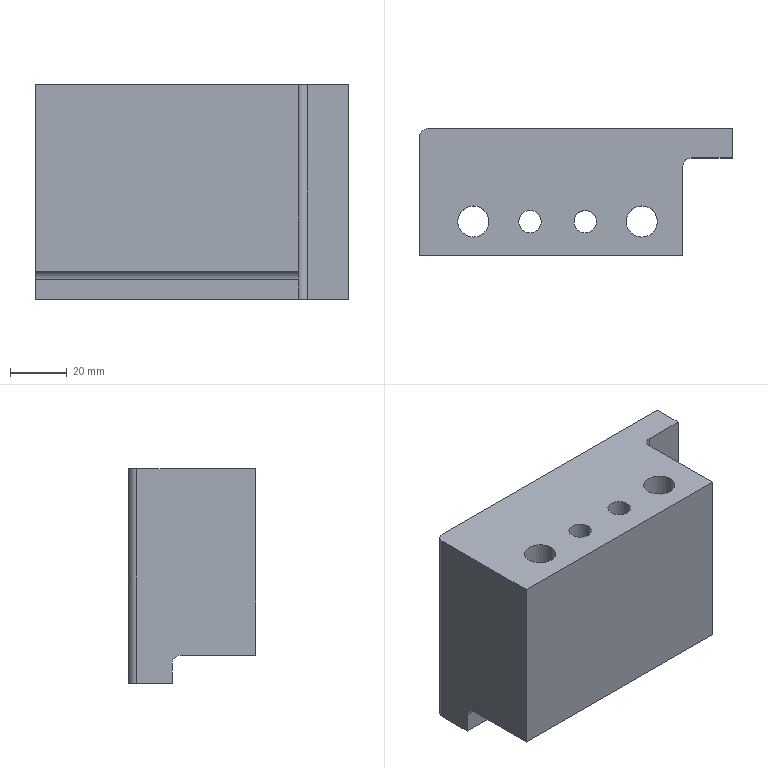Part | NX | features solid 2 | 1 solid | 25 faces | box 110.531 x 45 x 76 mm | volume 273418 mm3 | plane 14 | cylinder 11 | commonest cylinder face diameters 6 x3 8 x2 10.505 x2 11 x2 17 x2
STEP:
#1=CARTESIAN_POINT('',(667.977,-186.119,32.999));
#2=VERTEX_POINT('',#1);
#3=CARTESIAN_POINT('',(667.977,-180.619,32.999));
#4=DIRECTION('',(0.000000053,-0.000000517,1.));
#5=DIRECTION('',(0.,-1.,-0.000000517));
#6=AXIS2_PLACEMENT_3D('',#3,#4,#5);
#7=CIRCLE('',#6,5.5);
#8=EDGE_CURVE('',#2,#2,#7,.F.);
#9=ORIENTED_EDGE('',*,*,#8,.T.);
#10=EDGE_LOOP('',(#9));
#11=FACE_BOUND('',#10,.T.);
#12=CARTESIAN_POINT('',(647.977,-184.619,32.999));
#13=VERTEX_POINT('',#12);
#14=CARTESIAN_POINT('',(647.977,-180.619,32.999));
#15=DIRECTION('',(-0.000000053,0.000000517,-1.));
#16=DIRECTION('',(0.,-1.,-0.000000517));
#17=AXIS2_PLACEMENT_3D('',#14,#15,#16);
#18=CIRCLE('',#17,4.);
#19=EDGE_CURVE('',#13,#13,#18,.T.);
#20=ORIENTED_EDGE('',*,*,#19,.T.);
#21=EDGE_LOOP('',(#20));
#22=FACE_BOUND('',#21,.T.);
#23=CARTESIAN_POINT('',(628.446,-184.619,32.999));
#24=VERTEX_POINT('',#23);
#25=CARTESIAN_POINT('',(628.446,-180.619,32.999));
#26=DIRECTION('',(-0.000000053,0.000000517,-1.));
#27=DIRECTION('',(0.,-1.,-0.000000517));
#28=AXIS2_PLACEMENT_3D('',#25,#26,#27);
#29=CIRCLE('',#28,4.);
#30=EDGE_CURVE('',#24,#24,#29,.T.);
#31=ORIENTED_EDGE('',*,*,#30,.T.);
#32=EDGE_LOOP('',(#31));
#33=FACE_BOUND('',#32,.T.);
#34=CARTESIAN_POINT('',(608.446,-186.119,32.999));
#35=VERTEX_POINT('',#34);
#36=CARTESIAN_POINT('',(608.446,-180.619,32.999));
#37=DIRECTION('',(0.000000053,-0.000000517,1.));
#38=DIRECTION('',(0.,-1.,-0.000000517));
#39=AXIS2_PLACEMENT_3D('',#36,#37,#38);
#40=CIRCLE('',#39,5.5);
#41=EDGE_CURVE('',#35,#35,#40,.F.);
#42=ORIENTED_EDGE('',*,*,#41,.T.);
#43=EDGE_LOOP('',(#42));
#44=FACE_BOUND('',#43,.T.);
#45=CARTESIAN_POINT('',(682.498,-161.1,32.999));
#46=VERTEX_POINT('',#45);
#47=CARTESIAN_POINT('',(682.498,-192.619,32.999));
#48=VERTEX_POINT('',#47);
#49=CARTESIAN_POINT('',(682.498,-187.619,32.999));
#50=DIRECTION('',(0.,1.,0.000000517));
#51=VECTOR('',#50,1000.);
#52=LINE('',#49,#51);
#53=EDGE_CURVE('',#46,#48,#52,.F.);
#54=ORIENTED_EDGE('',*,*,#53,.F.);
#55=CARTESIAN_POINT('',(685.498,-158.1,32.999));
#56=VERTEX_POINT('',#55);
#57=CARTESIAN_POINT('',(685.498,-161.1,32.999));
#58=DIRECTION('',(0.000000053,-0.000000517,1.));
#59=DIRECTION('',(-0.01202,0.9999,0.000000518));
#60=AXIS2_PLACEMENT_3D('',#57,#58,#59);
#61=ELLIPSE('',#60,3.,3.);
#62=EDGE_CURVE('',#46,#56,#61,.F.);
#63=ORIENTED_EDGE('',*,*,#62,.T.);
#64=CARTESIAN_POINT('',(699.977,-158.1,32.999));
#65=VERTEX_POINT('',#64);
#66=CARTESIAN_POINT('',(699.977,-158.1,32.999));
#67=DIRECTION('',(-1.,0.,0.000000053));
#68=VECTOR('',#67,1000.);
#69=LINE('',#66,#68);
#70=EDGE_CURVE('',#65,#56,#69,.T.);
#71=ORIENTED_EDGE('',*,*,#70,.F.);
#72=CARTESIAN_POINT('',(699.977,-147.619,32.999));
#73=VERTEX_POINT('',#72);
#74=CARTESIAN_POINT('',(699.977,-187.619,32.999));
#75=DIRECTION('',(0.,1.,0.000000517));
#76=VECTOR('',#75,1000.);
#77=LINE('',#74,#76);
#78=EDGE_CURVE('',#65,#73,#77,.T.);
#79=ORIENTED_EDGE('',*,*,#78,.T.);
#80=CARTESIAN_POINT('',(592.446,-147.619,32.999));
#81=VERTEX_POINT('',#80);
#82=CARTESIAN_POINT('',(699.977,-147.619,32.999));
#83=DIRECTION('',(-1.,0.,0.000000053));
#84=VECTOR('',#83,1000.);
#85=LINE('',#82,#84);
#86=EDGE_CURVE('',#81,#73,#85,.F.);
#87=ORIENTED_EDGE('',*,*,#86,.F.);
#88=CARTESIAN_POINT('',(589.446,-150.619,32.999));
#89=VERTEX_POINT('',#88);
#90=CARTESIAN_POINT('',(592.446,-150.619,32.999));
#91=DIRECTION('',(0.000000053,-0.000000517,1.));
#92=DIRECTION('',(0.,1.,0.000000517));
#93=AXIS2_PLACEMENT_3D('',#90,#91,#92);
#94=CIRCLE('',#93,3.);
#95=EDGE_CURVE('',#89,#81,#94,.F.);
#96=ORIENTED_EDGE('',*,*,#95,.F.);
#97=CARTESIAN_POINT('',(589.446,-192.619,32.999));
#98=VERTEX_POINT('',#97);
#99=CARTESIAN_POINT('',(589.446,-177.619,32.999));
#100=DIRECTION('',(0.,1.,0.000000517));
#101=VECTOR('',#100,1000.);
#102=LINE('',#99,#101);
#103=EDGE_CURVE('',#89,#98,#102,.F.);
#104=ORIENTED_EDGE('',*,*,#103,.T.);
#105=CARTESIAN_POINT('',(699.977,-192.619,32.999));
#106=DIRECTION('',(-1.,0.,0.000000053));
#107=VECTOR('',#106,1000.);
#108=LINE('',#105,#107);
#109=EDGE_CURVE('',#98,#48,#108,.F.);
#110=ORIENTED_EDGE('',*,*,#109,.T.);
#111=EDGE_LOOP('',(#54,#63,#71,#79,#87,#96,#104,#110));
#112=FACE_BOUND('',#111,.T.);
#113=CARTESIAN_POINT('',(699.977,-187.619,32.999));
#114=DIRECTION('',(0.000000053,-0.000000517,1.));
#115=DIRECTION('',(1.,0.,-0.000000053));
#116=AXIS2_PLACEMENT_3D('',#113,#114,#115);
#117=PLANE('',#116);
#118=ADVANCED_FACE('',(#11,#22,#33,#44,#112),#117,.T.);
#119=CARTESIAN_POINT('',(682.498,-163.1,-43.001));
#120=VERTEX_POINT('',#119);
#121=CARTESIAN_POINT('',(682.498,-163.1,-36.001));
#122=VERTEX_POINT('',#121);
#123=CARTESIAN_POINT('',(682.498,-163.1,-5.001));
#124=DIRECTION('',(0.,0.000003911,1.));
#125=VECTOR('',#124,1000.);
#126=LINE('',#123,#125);
#127=EDGE_CURVE('',#120,#122,#126,.T.);
#128=ORIENTED_EDGE('',*,*,#127,.T.);
#129=CARTESIAN_POINT('',(589.446,-163.1,-36.001));
#130=VERTEX_POINT('',#129);
#131=CARTESIAN_POINT('',(589.446,-163.1,-36.001));
#132=DIRECTION('',(1.,0.,-0.000000053));
#133=VECTOR('',#132,1000.);
#134=LINE('',#131,#133);
#135=EDGE_CURVE('',#122,#130,#134,.F.);
#136=ORIENTED_EDGE('',*,*,#135,.T.);
#137=CARTESIAN_POINT('',(589.446,-163.1,-43.001));
#138=VERTEX_POINT('',#137);
#139=CARTESIAN_POINT('',(589.446,-163.1,-5.001));
#140=DIRECTION('',(-0.000000053,-0.000003911,-1.));
#141=VECTOR('',#140,1000.);
#142=LINE('',#139,#141);
#143=EDGE_CURVE('',#130,#138,#142,.T.);
#144=ORIENTED_EDGE('',*,*,#143,.T.);
#145=CARTESIAN_POINT('',(574.977,-163.1,-43.001));
#146=DIRECTION('',(-1.,0.,0.000000053));
#147=VECTOR('',#146,1000.);
#148=LINE('',#145,#147);
#149=EDGE_CURVE('',#120,#138,#148,.T.);
#150=ORIENTED_EDGE('',*,*,#149,.F.);
#151=EDGE_LOOP('',(#128,#136,#144,#150));
#152=FACE_BOUND('',#151,.T.);
#153=CARTESIAN_POINT('',(704.737,-163.1,-5.001));
#154=DIRECTION('',(0.,-1.,0.000003911));
#155=DIRECTION('',(0.,-0.000003911,-1.));
#156=AXIS2_PLACEMENT_3D('',#153,#154,#155);
#157=PLANE('',#156);
#158=ADVANCED_FACE('',(#152),#157,.T.);
#159=ORIENTED_EDGE('',*,*,#86,.T.);
#160=CARTESIAN_POINT('',(699.977,-147.619,-43.001));
#161=VERTEX_POINT('',#160);
#162=CARTESIAN_POINT('',(699.977,-147.619,56.368));
#163=DIRECTION('',(0.000000053,-0.000000517,1.));
#164=VECTOR('',#163,1000.);
#165=LINE('',#162,#164);
#166=EDGE_CURVE('',#161,#73,#165,.T.);
#167=ORIENTED_EDGE('',*,*,#166,.F.);
#168=CARTESIAN_POINT('',(592.446,-147.619,-43.001));
#169=VERTEX_POINT('',#168);
#170=CARTESIAN_POINT('',(574.977,-147.619,-43.001));
#171=DIRECTION('',(1.,0.,-0.000000053));
#172=VECTOR('',#171,1000.);
#173=LINE('',#170,#172);
#174=EDGE_CURVE('',#169,#161,#173,.T.);
#175=ORIENTED_EDGE('',*,*,#174,.F.);
#176=CARTESIAN_POINT('',(592.446,-147.619,56.368));
#177=DIRECTION('',(-0.000000053,0.000000517,-1.));
#178=VECTOR('',#177,1000.);
#179=LINE('',#176,#178);
#180=EDGE_CURVE('',#81,#169,#179,.T.);
#181=ORIENTED_EDGE('',*,*,#180,.F.);
#182=EDGE_LOOP('',(#159,#167,#175,#181));
#183=FACE_BOUND('',#182,.T.);
#184=CARTESIAN_POINT('',(583.446,-147.619,56.368));
#185=DIRECTION('',(0.,-1.,-0.000000517));
#186=DIRECTION('',(-0.000000053,0.000000517,-1.));
#187=AXIS2_PLACEMENT_3D('',#184,#185,#186);
#188=PLANE('',#187);
#189=ADVANCED_FACE('',(#183),#188,.F.);
#190=ORIENTED_EDGE('',*,*,#174,.T.);
#191=CARTESIAN_POINT('',(699.977,-158.1,-43.001));
#192=VERTEX_POINT('',#191);
#193=CARTESIAN_POINT('',(699.977,-110.331,-43.001));
#194=DIRECTION('',(0.,-1.,-0.000000517));
#195=VECTOR('',#194,1000.);
#196=LINE('',#193,#195);
#197=EDGE_CURVE('',#161,#192,#196,.T.);
#198=ORIENTED_EDGE('',*,*,#197,.T.);
#199=CARTESIAN_POINT('',(685.498,-158.1,-43.001));
#200=VERTEX_POINT('',#199);
#201=CARTESIAN_POINT('',(574.977,-158.1,-43.001));
#202=DIRECTION('',(-1.,0.,0.000000053));
#203=VECTOR('',#202,1000.);
#204=LINE('',#201,#203);
#205=EDGE_CURVE('',#192,#200,#204,.T.);
#206=ORIENTED_EDGE('',*,*,#205,.T.);
#207=CARTESIAN_POINT('',(682.498,-161.1,-43.001));
#208=VERTEX_POINT('',#207);
#209=CARTESIAN_POINT('',(685.498,-161.1,-43.001));
#210=DIRECTION('',(-0.000000053,0.000000517,-1.));
#211=DIRECTION('',(-0.01202,0.9999,0.000000518));
#212=AXIS2_PLACEMENT_3D('',#209,#210,#211);
#213=ELLIPSE('',#212,3.,3.);
#214=EDGE_CURVE('',#200,#208,#213,.F.);
#215=ORIENTED_EDGE('',*,*,#214,.T.);
#216=CARTESIAN_POINT('',(682.498,-110.331,-43.001));
#217=DIRECTION('',(0.,-1.,-0.000000517));
#218=VECTOR('',#217,1000.);
#219=LINE('',#216,#218);
#220=EDGE_CURVE('',#208,#120,#219,.T.);
#221=ORIENTED_EDGE('',*,*,#220,.T.);
#222=ORIENTED_EDGE('',*,*,#149,.T.);
#223=CARTESIAN_POINT('',(589.446,-150.619,-43.001));
#224=VERTEX_POINT('',#223);
#225=CARTESIAN_POINT('',(589.446,-110.331,-43.001));
#226=DIRECTION('',(0.,1.,0.000000517));
#227=VECTOR('',#226,1000.);
#228=LINE('',#225,#227);
#229=EDGE_CURVE('',#138,#224,#228,.T.);
#230=ORIENTED_EDGE('',*,*,#229,.T.);
#231=CARTESIAN_POINT('',(592.446,-150.619,-43.001));
#232=DIRECTION('',(-0.000000053,0.000000517,-1.));
#233=DIRECTION('',(0.,-1.,-0.000000517));
#234=AXIS2_PLACEMENT_3D('',#231,#232,#233);
#235=CIRCLE('',#234,3.);
#236=EDGE_CURVE('',#169,#224,#235,.F.);
#237=ORIENTED_EDGE('',*,*,#236,.F.);
#238=EDGE_LOOP('',(#190,#198,#206,#215,#221,#222,#230,#237));
#239=FACE_BOUND('',#238,.T.);
#240=CARTESIAN_POINT('',(574.977,-110.331,-43.001));
#241=DIRECTION('',(-0.000000053,0.000000517,-1.));
#242=DIRECTION('',(1.,0.,-0.000000053));
#243=AXIS2_PLACEMENT_3D('',#240,#241,#242);
#244=PLANE('',#243);
#245=ADVANCED_FACE('',(#239),#244,.T.);
#246=CARTESIAN_POINT('',(589.446,-192.619,-33.001));
#247=VERTEX_POINT('',#246);
#248=CARTESIAN_POINT('',(589.446,-166.1,-33.001));
#249=VERTEX_POINT('',#248);
#250=CARTESIAN_POINT('',(589.446,-110.331,-33.001));
#251=DIRECTION('',(0.,1.,0.000000517));
#252=VECTOR('',#251,1000.);
#253=LINE('',#250,#252);
#254=EDGE_CURVE('',#247,#249,#253,.T.);
#255=ORIENTED_EDGE('',*,*,#254,.T.);
#256=CARTESIAN_POINT('',(682.498,-166.1,-33.001));
#257=VERTEX_POINT('',#256);
#258=CARTESIAN_POINT('',(682.498,-166.1,-33.001));
#259=DIRECTION('',(1.,0.,-0.000000053));
#260=VECTOR('',#259,1000.);
#261=LINE('',#258,#260);
#262=EDGE_CURVE('',#249,#257,#261,.T.);
#263=ORIENTED_EDGE('',*,*,#262,.T.);
#264=CARTESIAN_POINT('',(682.498,-192.619,-33.001));
#265=VERTEX_POINT('',#264);
#266=CARTESIAN_POINT('',(682.498,-110.331,-33.001));
#267=DIRECTION('',(0.,-1.,-0.000000517));
#268=VECTOR('',#267,1000.);
#269=LINE('',#266,#268);
#270=EDGE_CURVE('',#257,#265,#269,.T.);
#271=ORIENTED_EDGE('',*,*,#270,.T.);
#272=CARTESIAN_POINT('',(574.977,-192.619,-33.001));
#273=DIRECTION('',(-1.,0.,0.000000053));
#274=VECTOR('',#273,1000.);
#275=LINE('',#272,#274);
#276=EDGE_CURVE('',#265,#247,#275,.T.);
#277=ORIENTED_EDGE('',*,*,#276,.T.);
#278=EDGE_LOOP('',(#255,#263,#271,#277));
#279=FACE_BOUND('',#278,.T.);
#280=CARTESIAN_POINT('',(608.446,-172.119,-33.001));
#281=VERTEX_POINT('',#280);
#282=CARTESIAN_POINT('',(608.446,-180.619,-33.001));
#283=DIRECTION('',(-0.000000053,0.000000517,-1.));
#284=DIRECTION('',(0.,1.,0.000000517));
#285=AXIS2_PLACEMENT_3D('',#282,#283,#284);
#286=CIRCLE('',#285,8.5);
#287=EDGE_CURVE('',#281,#281,#286,.T.);
#288=ORIENTED_EDGE('',*,*,#287,.F.);
#289=EDGE_LOOP('',(#288));
#290=FACE_BOUND('',#289,.T.);
#291=CARTESIAN_POINT('',(628.446,-175.366,-33.001));
#292=VERTEX_POINT('',#291);
#293=CARTESIAN_POINT('',(627.378,-175.439,-33.001));
#294=CARTESIAN_POINT('',(628.411,-175.332,-33.001));
#295=CARTESIAN_POINT('',(629.442,-175.429,-33.001));
#296=CARTESIAN_POINT('',(630.419,-175.714,-33.001));
#297=CARTESIAN_POINT('',(631.337,-176.193,-33.001));
#298=CARTESIAN_POINT('',(632.145,-176.842,-33.001));
#299=CARTESIAN_POINT('',(632.811,-177.636,-33.001));
#300=CARTESIAN_POINT('',(633.309,-178.545,-33.001));
#301=CARTESIAN_POINT('',(633.62,-179.533,-33.001));
#302=CARTESIAN_POINT('',(633.732,-180.564,-33.001));
#303=CARTESIAN_POINT('',(633.641,-181.596,-33.001));
#304=CARTESIAN_POINT('',(633.351,-182.591,-33.001));
#305=CARTESIAN_POINT('',(632.872,-183.51,-33.001));
#306=CARTESIAN_POINT('',(632.223,-184.318,-33.001));
#307=CARTESIAN_POINT('',(631.428,-184.983,-33.001));
#308=CARTESIAN_POINT('',(630.52,-185.481,-33.001));
#309=CARTESIAN_POINT('',(629.531,-185.792,-33.001));
#310=CARTESIAN_POINT('',(628.501,-185.905,-33.001));
#311=CARTESIAN_POINT('',(627.469,-185.814,-33.001));
#312=CARTESIAN_POINT('',(626.474,-185.523,-33.001));
#313=CARTESIAN_POINT('',(625.555,-185.044,-33.001));
#314=CARTESIAN_POINT('',(624.747,-184.395,-33.001));
#315=CARTESIAN_POINT('',(624.081,-183.601,-33.001));
#316=CARTESIAN_POINT('',(623.583,-182.692,-33.001));
#317=CARTESIAN_POINT('',(623.272,-181.704,-33.001));
#318=CARTESIAN_POINT('',(623.16,-180.673,-33.001));
#319=CARTESIAN_POINT('',(623.251,-179.641,-33.001));
#320=CARTESIAN_POINT('',(623.541,-178.646,-33.001));
#321=CARTESIAN_POINT('',(624.02,-177.727,-33.001));
#322=CARTESIAN_POINT('',(624.669,-176.919,-33.001));
#323=CARTESIAN_POINT('',(625.464,-176.254,-33.001));
#324=CARTESIAN_POINT('',(626.373,-175.756,-33.001));
#325=CARTESIAN_POINT('',(627.378,-175.439,-33.001));
#326=CARTESIAN_POINT('',(628.411,-175.332,-33.001));
#327=CARTESIAN_POINT('',(629.442,-175.429,-33.001));
#328=B_SPLINE_CURVE_WITH_KNOTS('',3,(#293,#294,#295,#296,#297,#298,#299,#300,#301,#302,#303,#304,#305,#306,#307,#308,#309,#310,#311,#312,#313,#314,#315,#316,#317,#318,#319,#320,#321,#322,#323,#324,#325,#326,#327),.UNSPECIFIED.,.T.,.F.,(1,1,1,1,1,1,1,1,1,1,1,1,1,1,1,1,1,1,1,1,1,1,1,1,1,1,1,1,1,1,1,1,1,1,1,1,1,1,1),(-0.09539,-0.06414,-0.03289,0.,0.02969,0.06086,0.09211,0.1234,0.1546,0.1859,0.2171,0.2484,0.2796,0.3109,0.3421,0.3734,0.4046,0.4359,0.4671,0.4984,0.5296,0.5609,0.5921,0.6234,0.6546,0.6859,0.7171,0.7484,0.7796,0.8109,0.8421,0.8734,0.9046,0.9359,0.9671,1.,1.03,1.061,1.092),.UNSPECIFIED.);
#329=EDGE_CURVE('',#292,#292,#328,.T.);
#330=ORIENTED_EDGE('',*,*,#329,.F.);
#331=EDGE_LOOP('',(#330));
#332=FACE_BOUND('',#331,.T.);
#333=CARTESIAN_POINT('',(647.977,-175.366,-33.001));
#334=VERTEX_POINT('',#333);
#335=CARTESIAN_POINT('',(649.045,-175.439,-33.001));
#336=CARTESIAN_POINT('',(648.012,-175.332,-33.001));
#337=CARTESIAN_POINT('',(646.981,-175.429,-33.001));
#338=CARTESIAN_POINT('',(646.004,-175.714,-33.001));
#339=CARTESIAN_POINT('',(645.086,-176.193,-33.001));
#340=CARTESIAN_POINT('',(644.278,-176.842,-33.001));
#341=CARTESIAN_POINT('',(643.613,-177.636,-33.001));
#342=CARTESIAN_POINT('',(643.115,-178.545,-33.001));
#343=CARTESIAN_POINT('',(642.804,-179.533,-33.001));
#344=CARTESIAN_POINT('',(642.691,-180.564,-33.001));
#345=CARTESIAN_POINT('',(642.782,-181.596,-33.001));
#346=CARTESIAN_POINT('',(643.073,-182.591,-33.001));
#347=CARTESIAN_POINT('',(643.552,-183.51,-33.001));
#348=CARTESIAN_POINT('',(644.201,-184.318,-33.001));
#349=CARTESIAN_POINT('',(644.995,-184.983,-33.001));
#350=CARTESIAN_POINT('',(645.904,-185.481,-33.001));
#351=CARTESIAN_POINT('',(646.892,-185.792,-33.001));
#352=CARTESIAN_POINT('',(647.923,-185.905,-33.001));
#353=CARTESIAN_POINT('',(648.955,-185.814,-33.001));
#354=CARTESIAN_POINT('',(649.95,-185.523,-33.001));
#355=CARTESIAN_POINT('',(650.869,-185.044,-33.001));
#356=CARTESIAN_POINT('',(651.676,-184.395,-33.001));
#357=CARTESIAN_POINT('',(652.342,-183.601,-33.001));
#358=CARTESIAN_POINT('',(652.84,-182.692,-33.001));
#359=CARTESIAN_POINT('',(653.151,-181.703,-33.001));
#360=CARTESIAN_POINT('',(653.263,-180.673,-33.001));
#361=CARTESIAN_POINT('',(653.173,-179.641,-33.001));
#362=CARTESIAN_POINT('',(652.882,-178.646,-33.001));
#363=CARTESIAN_POINT('',(652.403,-177.727,-33.001));
#364=CARTESIAN_POINT('',(651.754,-176.919,-33.001));
#365=CARTESIAN_POINT('',(650.96,-176.254,-33.001));
#366=CARTESIAN_POINT('',(650.051,-175.756,-33.001));
#367=CARTESIAN_POINT('',(649.045,-175.439,-33.001));
#368=CARTESIAN_POINT('',(648.012,-175.332,-33.001));
#369=CARTESIAN_POINT('',(646.981,-175.429,-33.001));
#370=B_SPLINE_CURVE_WITH_KNOTS('',3,(#335,#336,#337,#338,#339,#340,#341,#342,#343,#344,#345,#346,#347,#348,#349,#350,#351,#352,#353,#354,#355,#356,#357,#358,#359,#360,#361,#362,#363,#364,#365,#366,#367,#368,#369),.UNSPECIFIED.,.T.,.F.,(1,1,1,1,1,1,1,1,1,1,1,1,1,1,1,1,1,1,1,1,1,1,1,1,1,1,1,1,1,1,1,1,1,1,1,1,1,1,1),(-0.09539,-0.06414,-0.03289,0.,0.02969,0.06086,0.09211,0.1234,0.1546,0.1859,0.2171,0.2484,0.2796,0.3109,0.3421,0.3734,0.4046,0.4359,0.4671,0.4984,0.5296,0.5609,0.5921,0.6234,0.6546,0.6859,0.7171,0.7484,0.7796,0.8109,0.8421,0.8734,0.9046,0.9359,0.9671,1.,1.03,1.061,1.092),.UNSPECIFIED.);
#371=EDGE_CURVE('',#334,#334,#370,.F.);
#372=ORIENTED_EDGE('',*,*,#371,.F.);
#373=EDGE_LOOP('',(#372));
#374=FACE_BOUND('',#373,.T.);
#375=CARTESIAN_POINT('',(667.977,-172.119,-33.001));
#376=VERTEX_POINT('',#375);
#377=CARTESIAN_POINT('',(667.977,-180.619,-33.001));
#378=DIRECTION('',(-0.000000053,0.000000517,-1.));
#379=DIRECTION('',(0.,1.,0.000000517));
#380=AXIS2_PLACEMENT_3D('',#377,#378,#379);
#381=CIRCLE('',#380,8.5);
#382=EDGE_CURVE('',#376,#376,#381,.T.);
#383=ORIENTED_EDGE('',*,*,#382,.F.);
#384=EDGE_LOOP('',(#383));
#385=FACE_BOUND('',#384,.T.);
#386=CARTESIAN_POINT('',(574.977,-110.331,-33.001));
#387=DIRECTION('',(-0.000000053,0.000000517,-1.));
#388=DIRECTION('',(1.,0.,-0.000000053));
#389=AXIS2_PLACEMENT_3D('',#386,#387,#388);
#390=PLANE('',#389);
#391=ADVANCED_FACE('',(#279,#290,#332,#374,#385),#390,.T.);
#392=ORIENTED_EDGE('',*,*,#276,.F.);
#393=CARTESIAN_POINT('',(682.498,-192.619,-43.001));
#394=DIRECTION('',(0.,-0.000000517,1.));
#395=VECTOR('',#394,1000.);
#396=LINE('',#393,#395);
#397=EDGE_CURVE('',#265,#48,#396,.T.);
#398=ORIENTED_EDGE('',*,*,#397,.T.);
#399=ORIENTED_EDGE('',*,*,#109,.F.);
#400=CARTESIAN_POINT('',(589.446,-192.619,-43.001));
#401=DIRECTION('',(0.000000053,-0.000000517,1.));
#402=VECTOR('',#401,1000.);
#403=LINE('',#400,#402);
#404=EDGE_CURVE('',#98,#247,#403,.F.);
#405=ORIENTED_EDGE('',*,*,#404,.T.);
#406=EDGE_LOOP('',(#392,#398,#399,#405));
#407=FACE_BOUND('',#406,.T.);
#408=CARTESIAN_POINT('',(699.977,-192.619,-43.001));
#409=DIRECTION('',(0.,-1.,-0.000000517));
#410=DIRECTION('',(-0.000000053,0.000000517,-1.));
#411=AXIS2_PLACEMENT_3D('',#408,#409,#410);
#412=PLANE('',#411);
#413=ADVANCED_FACE('',(#407),#412,.T.);
#414=ORIENTED_EDGE('',*,*,#254,.F.);
#415=ORIENTED_EDGE('',*,*,#404,.F.);
#416=ORIENTED_EDGE('',*,*,#103,.F.);
#417=CARTESIAN_POINT('',(589.446,-150.619,-43.001));
#418=DIRECTION('',(-0.000000053,0.000000517,-1.));
#419=VECTOR('',#418,1000.);
#420=LINE('',#417,#419);
#421=EDGE_CURVE('',#224,#89,#420,.F.);
#422=ORIENTED_EDGE('',*,*,#421,.F.);
#423=ORIENTED_EDGE('',*,*,#229,.F.);
#424=ORIENTED_EDGE('',*,*,#143,.F.);
#425=CARTESIAN_POINT('',(589.446,-166.1,-36.001));
#426=DIRECTION('',(-1.,0.,0.000000053));
#427=DIRECTION('',(0.000000053,0.,1.));
#428=AXIS2_PLACEMENT_3D('',#425,#426,#427);
#429=CIRCLE('',#428,3.);
#430=EDGE_CURVE('',#130,#249,#429,.F.);
#431=ORIENTED_EDGE('',*,*,#430,.T.);
#432=EDGE_LOOP('',(#414,#415,#416,#422,#423,#424,#431));
#433=FACE_BOUND('',#432,.T.);
#434=CARTESIAN_POINT('',(589.446,-177.619,-43.001));
#435=DIRECTION('',(-1.,0.,0.000000053));
#436=DIRECTION('',(-0.000000053,0.000000517,-1.));
#437=AXIS2_PLACEMENT_3D('',#434,#435,#436);
#438=PLANE('',#437);
#439=ADVANCED_FACE('',(#433),#438,.T.);
#440=ORIENTED_EDGE('',*,*,#220,.F.);
#441=CARTESIAN_POINT('',(682.498,-161.1,32.999));
#442=DIRECTION('',(0.,-0.000003911,-1.));
#443=VECTOR('',#442,1000.);
#444=LINE('',#441,#443);
#445=EDGE_CURVE('',#208,#46,#444,.F.);
#446=ORIENTED_EDGE('',*,*,#445,.T.);
#447=ORIENTED_EDGE('',*,*,#53,.T.);
#448=ORIENTED_EDGE('',*,*,#397,.F.);
#449=ORIENTED_EDGE('',*,*,#270,.F.);
#450=CARTESIAN_POINT('',(682.498,-166.1,-36.001));
#451=DIRECTION('',(1.,0.,0.));
#452=DIRECTION('',(0.,1.,0.));
#453=AXIS2_PLACEMENT_3D('',#450,#451,#452);
#454=CIRCLE('',#453,3.);
#455=EDGE_CURVE('',#257,#122,#454,.F.);
#456=ORIENTED_EDGE('',*,*,#455,.T.);
#457=ORIENTED_EDGE('',*,*,#127,.F.);
#458=EDGE_LOOP('',(#440,#446,#447,#448,#449,#456,#457));
#459=FACE_BOUND('',#458,.T.);
#460=CARTESIAN_POINT('',(682.498,-177.1,49.2));
#461=DIRECTION('',(1.,0.,0.));
#462=DIRECTION('',(0.,1.,-0.000003329));
#463=AXIS2_PLACEMENT_3D('',#460,#461,#462);
#464=PLANE('',#463);
#465=ADVANCED_FACE('',(#459),#464,.T.);
#466=CARTESIAN_POINT('',(667.977,-175.119,7.999));
#467=VERTEX_POINT('',#466);
#468=CARTESIAN_POINT('',(667.977,-180.619,7.999));
#469=DIRECTION('',(-0.000000053,0.000000517,-1.));
#470=DIRECTION('',(0.,1.,0.000000517));
#471=AXIS2_PLACEMENT_3D('',#468,#469,#470);
#472=CIRCLE('',#471,5.5);
#473=EDGE_CURVE('',#467,#467,#472,.T.);
#474=ORIENTED_EDGE('',*,*,#473,.T.);
#475=EDGE_LOOP('',(#474));
#476=FACE_BOUND('',#475,.T.);
#477=ORIENTED_EDGE('',*,*,#8,.F.);
#478=EDGE_LOOP('',(#477));
#479=FACE_BOUND('',#478,.T.);
#480=CARTESIAN_POINT('',(667.977,-180.619,33.999));
#481=DIRECTION('',(-0.000000053,0.000000517,-1.));
#482=DIRECTION('',(0.,-1.,-0.000000517));
#483=AXIS2_PLACEMENT_3D('',#480,#481,#482);
#484=CYLINDRICAL_SURFACE('',#483,5.5);
#485=ADVANCED_FACE('',(#476,#479),#484,.F.);
#486=ORIENTED_EDGE('',*,*,#382,.T.);
#487=EDGE_LOOP('',(#486));
#488=FACE_BOUND('',#487,.T.);
#489=CARTESIAN_POINT('',(667.977,-172.119,7.999));
#490=VERTEX_POINT('',#489);
#491=CARTESIAN_POINT('',(667.977,-180.619,7.999));
#492=DIRECTION('',(-0.000000053,0.000000517,-1.));
#493=DIRECTION('',(0.,1.,0.000000517));
#494=AXIS2_PLACEMENT_3D('',#491,#492,#493);
#495=CIRCLE('',#494,8.5);
#496=EDGE_CURVE('',#490,#490,#495,.F.);
#497=ORIENTED_EDGE('',*,*,#496,.T.);
#498=EDGE_LOOP('',(#497));
#499=FACE_BOUND('',#498,.T.);
#500=CARTESIAN_POINT('',(667.977,-180.619,7.999));
#501=DIRECTION('',(-0.000000053,0.000000517,-1.));
#502=DIRECTION('',(0.,-1.,-0.000000517));
#503=AXIS2_PLACEMENT_3D('',#500,#501,#502);
#504=CYLINDRICAL_SURFACE('',#503,8.5);
#505=ADVANCED_FACE('',(#488,#499),#504,.F.);
#506=ORIENTED_EDGE('',*,*,#473,.F.);
#507=EDGE_LOOP('',(#506));
#508=FACE_BOUND('',#507,.T.);
#509=ORIENTED_EDGE('',*,*,#496,.F.);
#510=EDGE_LOOP('',(#509));
#511=FACE_BOUND('',#510,.T.);
#512=CARTESIAN_POINT('',(667.977,-180.619,7.999));
#513=DIRECTION('',(-0.000000053,0.000000517,-1.));
#514=DIRECTION('',(0.,-1.,-0.000000517));
#515=AXIS2_PLACEMENT_3D('',#512,#513,#514);
#516=PLANE('',#515);
#517=ADVANCED_FACE('',(#508,#511),#516,.T.);
#518=CARTESIAN_POINT('',(651.977,-180.618,-13.001));
#519=VERTEX_POINT('',#518);
#520=CARTESIAN_POINT('',(647.977,-180.618,-13.001));
#521=DIRECTION('',(-0.000000981,-0.000001551,1.));
#522=DIRECTION('',(1.,0.,0.000000981));
#523=AXIS2_PLACEMENT_3D('',#520,#521,#522);
#524=CIRCLE('',#523,4.);
#525=EDGE_CURVE('',#519,#519,#524,.F.);
#526=ORIENTED_EDGE('',*,*,#525,.T.);
#527=EDGE_LOOP('',(#526));
#528=FACE_BOUND('',#527,.T.);
#529=ORIENTED_EDGE('',*,*,#19,.F.);
#530=EDGE_LOOP('',(#529));
#531=FACE_BOUND('',#530,.T.);
#532=CARTESIAN_POINT('',(647.977,-180.619,33.999));
#533=DIRECTION('',(0.000000981,0.000001551,-1.));
#534=DIRECTION('',(0.,-1.,-0.000001551));
#535=AXIS2_PLACEMENT_3D('',#532,#533,#534);
#536=CYLINDRICAL_SURFACE('',#535,4.);
#537=ADVANCED_FACE('',(#528,#531),#536,.F.);
#538=ORIENTED_EDGE('',*,*,#371,.T.);
#539=EDGE_LOOP('',(#538));
#540=FACE_BOUND('',#539,.T.);
#541=CARTESIAN_POINT('',(653.23,-180.618,-13.001));
#542=VERTEX_POINT('',#541);
#543=CARTESIAN_POINT('',(647.977,-180.618,-13.001));
#544=DIRECTION('',(-0.000000981,-0.000001551,1.));
#545=DIRECTION('',(1.,0.,0.000000981));
#546=AXIS2_PLACEMENT_3D('',#543,#544,#545);
#547=CIRCLE('',#546,5.253);
#548=EDGE_CURVE('',#542,#542,#547,.T.);
#549=ORIENTED_EDGE('',*,*,#548,.T.);
#550=EDGE_LOOP('',(#549));
#551=FACE_BOUND('',#550,.T.);
#552=CARTESIAN_POINT('',(647.977,-180.618,-33.001));
#553=DIRECTION('',(0.000000981,0.000001551,-1.));
#554=DIRECTION('',(0.,-1.,-0.000001551));
#555=AXIS2_PLACEMENT_3D('',#552,#553,#554);
#556=CYLINDRICAL_SURFACE('',#555,5.253);
#557=ADVANCED_FACE('',(#540,#551),#556,.F.);
#558=ORIENTED_EDGE('',*,*,#525,.F.);
#559=EDGE_LOOP('',(#558));
#560=FACE_BOUND('',#559,.T.);
#561=ORIENTED_EDGE('',*,*,#548,.F.);
#562=EDGE_LOOP('',(#561));
#563=FACE_BOUND('',#562,.T.);
#564=CARTESIAN_POINT('',(647.977,-180.618,-13.001));
#565=DIRECTION('',(0.000000981,0.000001551,-1.));
#566=DIRECTION('',(0.,-1.,-0.000001551));
#567=AXIS2_PLACEMENT_3D('',#564,#565,#566);
#568=PLANE('',#567);
#569=ADVANCED_FACE('',(#560,#563),#568,.T.);
#570=CARTESIAN_POINT('',(628.446,-184.619,-13.001));
#571=VERTEX_POINT('',#570);
#572=CARTESIAN_POINT('',(628.446,-180.619,-13.001));
#573=DIRECTION('',(0.000000981,-0.000001551,1.));
#574=DIRECTION('',(0.,-1.,-0.000001551));
#575=AXIS2_PLACEMENT_3D('',#572,#573,#574);
#576=CIRCLE('',#575,4.);
#577=EDGE_CURVE('',#571,#571,#576,.T.);
#578=ORIENTED_EDGE('',*,*,#577,.F.);
#579=EDGE_LOOP('',(#578));
#580=FACE_BOUND('',#579,.T.);
#581=ORIENTED_EDGE('',*,*,#30,.F.);
#582=EDGE_LOOP('',(#581));
#583=FACE_BOUND('',#582,.T.);
#584=CARTESIAN_POINT('',(628.446,-180.619,33.999));
#585=DIRECTION('',(-0.000000981,0.000001551,-1.));
#586=DIRECTION('',(0.,-1.,-0.000001551));
#587=AXIS2_PLACEMENT_3D('',#584,#585,#586);
#588=CYLINDRICAL_SURFACE('',#587,4.);
#589=ADVANCED_FACE('',(#580,#583),#588,.F.);
#590=ORIENTED_EDGE('',*,*,#329,.T.);
#591=EDGE_LOOP('',(#590));
#592=FACE_BOUND('',#591,.T.);
#593=CARTESIAN_POINT('',(623.194,-180.619,-13.001));
#594=VERTEX_POINT('',#593);
#595=CARTESIAN_POINT('',(628.446,-180.619,-13.001));
#596=DIRECTION('',(0.000000981,-0.000001551,1.));
#597=DIRECTION('',(-1.,0.,0.000000981));
#598=AXIS2_PLACEMENT_3D('',#595,#596,#597);
#599=CIRCLE('',#598,5.253);
#600=EDGE_CURVE('',#594,#594,#599,.F.);
#601=ORIENTED_EDGE('',*,*,#600,.F.);
#602=EDGE_LOOP('',(#601));
#603=FACE_BOUND('',#602,.T.);
#604=CARTESIAN_POINT('',(628.446,-180.618,-33.001));
#605=DIRECTION('',(-0.000000981,0.000001551,-1.));
#606=DIRECTION('',(0.,-1.,-0.000001551));
#607=AXIS2_PLACEMENT_3D('',#604,#605,#606);
#608=CYLINDRICAL_SURFACE('',#607,5.253);
#609=ADVANCED_FACE('',(#592,#603),#608,.F.);
#610=ORIENTED_EDGE('',*,*,#577,.T.);
#611=EDGE_LOOP('',(#610));
#612=FACE_BOUND('',#611,.T.);
#613=ORIENTED_EDGE('',*,*,#600,.T.);
#614=EDGE_LOOP('',(#613));
#615=FACE_BOUND('',#614,.T.);
#616=CARTESIAN_POINT('',(628.446,-180.619,-13.001));
#617=DIRECTION('',(-0.000000981,0.000001551,-1.));
#618=DIRECTION('',(0.,-1.,-0.000001551));
#619=AXIS2_PLACEMENT_3D('',#616,#617,#618);
#620=PLANE('',#619);
#621=ADVANCED_FACE('',(#612,#615),#620,.T.);
#622=CARTESIAN_POINT('',(608.446,-175.119,7.999));
#623=VERTEX_POINT('',#622);
#624=CARTESIAN_POINT('',(608.446,-180.619,7.999));
#625=DIRECTION('',(0.000000053,0.000000517,-1.));
#626=DIRECTION('',(0.,1.,0.000000517));
#627=AXIS2_PLACEMENT_3D('',#624,#625,#626);
#628=CIRCLE('',#627,5.5);
#629=EDGE_CURVE('',#623,#623,#628,.F.);
#630=ORIENTED_EDGE('',*,*,#629,.F.);
#631=EDGE_LOOP('',(#630));
#632=FACE_BOUND('',#631,.T.);
#633=ORIENTED_EDGE('',*,*,#41,.F.);
#634=EDGE_LOOP('',(#633));
#635=FACE_BOUND('',#634,.T.);
#636=CARTESIAN_POINT('',(608.446,-180.619,33.999));
#637=DIRECTION('',(0.000000053,0.000000517,-1.));
#638=DIRECTION('',(0.,-1.,-0.000000517));
#639=AXIS2_PLACEMENT_3D('',#636,#637,#638);
#640=CYLINDRICAL_SURFACE('',#639,5.5);
#641=ADVANCED_FACE('',(#632,#635),#640,.F.);
#642=ORIENTED_EDGE('',*,*,#287,.T.);
#643=EDGE_LOOP('',(#642));
#644=FACE_BOUND('',#643,.T.);
#645=CARTESIAN_POINT('',(608.446,-172.119,7.999));
#646=VERTEX_POINT('',#645);
#647=CARTESIAN_POINT('',(608.446,-180.619,7.999));
#648=DIRECTION('',(0.000000053,0.000000517,-1.));
#649=DIRECTION('',(0.,1.,0.000000517));
#650=AXIS2_PLACEMENT_3D('',#647,#648,#649);
#651=CIRCLE('',#650,8.5);
#652=EDGE_CURVE('',#646,#646,#651,.T.);
#653=ORIENTED_EDGE('',*,*,#652,.F.);
#654=EDGE_LOOP('',(#653));
#655=FACE_BOUND('',#654,.T.);
#656=CARTESIAN_POINT('',(608.446,-180.619,7.999));
#657=DIRECTION('',(0.000000053,0.000000517,-1.));
#658=DIRECTION('',(0.,-1.,-0.000000517));
#659=AXIS2_PLACEMENT_3D('',#656,#657,#658);
#660=CYLINDRICAL_SURFACE('',#659,8.5);
#661=ADVANCED_FACE('',(#644,#655),#660,.F.);
#662=ORIENTED_EDGE('',*,*,#629,.T.);
#663=EDGE_LOOP('',(#662));
#664=FACE_BOUND('',#663,.T.);
#665=ORIENTED_EDGE('',*,*,#652,.T.);
#666=EDGE_LOOP('',(#665));
#667=FACE_BOUND('',#666,.T.);
#668=CARTESIAN_POINT('',(608.446,-180.619,7.999));
#669=DIRECTION('',(0.000000053,0.000000517,-1.));
#670=DIRECTION('',(0.,-1.,-0.000000517));
#671=AXIS2_PLACEMENT_3D('',#668,#669,#670);
#672=PLANE('',#671);
#673=ADVANCED_FACE('',(#664,#667),#672,.T.);
#674=ORIENTED_EDGE('',*,*,#95,.T.);
#675=ORIENTED_EDGE('',*,*,#180,.T.);
#676=ORIENTED_EDGE('',*,*,#236,.T.);
#677=ORIENTED_EDGE('',*,*,#421,.T.);
#678=EDGE_LOOP('',(#674,#675,#676,#677));
#679=FACE_BOUND('',#678,.T.);
#680=CARTESIAN_POINT('',(592.446,-150.619,56.368));
#681=DIRECTION('',(-0.000000053,0.000000517,-1.));
#682=DIRECTION('',(0.,-1.,-0.000000517));
#683=AXIS2_PLACEMENT_3D('',#680,#681,#682);
#684=CYLINDRICAL_SURFACE('',#683,3.);
#685=ADVANCED_FACE('',(#679),#684,.T.);
#686=ORIENTED_EDGE('',*,*,#197,.F.);
#687=ORIENTED_EDGE('',*,*,#166,.T.);
#688=ORIENTED_EDGE('',*,*,#78,.F.);
#689=CARTESIAN_POINT('',(699.977,-158.101,-70.8));
#690=DIRECTION('',(0.000000053,0.000003911,1.));
#691=VECTOR('',#690,1000.);
#692=LINE('',#689,#691);
#693=EDGE_CURVE('',#192,#65,#692,.T.);
#694=ORIENTED_EDGE('',*,*,#693,.F.);
#695=EDGE_LOOP('',(#686,#687,#688,#694));
#696=FACE_BOUND('',#695,.T.);
#697=CARTESIAN_POINT('',(699.977,-147.619,-43.001));
#698=DIRECTION('',(1.,0.,-0.000000053));
#699=DIRECTION('',(0.000000053,0.,1.));
#700=AXIS2_PLACEMENT_3D('',#697,#698,#699);
#701=PLANE('',#700);
#702=ADVANCED_FACE('',(#696),#701,.T.);
#703=ORIENTED_EDGE('',*,*,#70,.T.);
#704=CARTESIAN_POINT('',(685.498,-158.1,-43.001));
#705=DIRECTION('',(0.,-0.000003911,-1.));
#706=VECTOR('',#705,1000.);
#707=LINE('',#704,#706);
#708=EDGE_CURVE('',#56,#200,#707,.T.);
#709=ORIENTED_EDGE('',*,*,#708,.T.);
#710=ORIENTED_EDGE('',*,*,#205,.F.);
#711=ORIENTED_EDGE('',*,*,#693,.T.);
#712=EDGE_LOOP('',(#703,#709,#710,#711));
#713=FACE_BOUND('',#712,.T.);
#714=CARTESIAN_POINT('',(704.737,-158.1,-5.001));
#715=DIRECTION('',(0.,-1.,0.000003911));
#716=DIRECTION('',(0.,-0.000003911,-1.));
#717=AXIS2_PLACEMENT_3D('',#714,#715,#716);
#718=PLANE('',#717);
#719=ADVANCED_FACE('',(#713),#718,.T.);
#720=ORIENTED_EDGE('',*,*,#62,.F.);
#721=ORIENTED_EDGE('',*,*,#445,.F.);
#722=ORIENTED_EDGE('',*,*,#214,.F.);
#723=ORIENTED_EDGE('',*,*,#708,.F.);
#724=EDGE_LOOP('',(#720,#721,#722,#723));
#725=FACE_BOUND('',#724,.T.);
#726=CARTESIAN_POINT('',(685.498,-161.1,-5.001));
#727=DIRECTION('',(0.,0.000003911,1.));
#728=DIRECTION('',(0.,-1.,0.000003911));
#729=AXIS2_PLACEMENT_3D('',#726,#727,#728);
#730=CYLINDRICAL_SURFACE('',#729,3.);
#731=ADVANCED_FACE('',(#725),#730,.F.);
#732=ORIENTED_EDGE('',*,*,#430,.F.);
#733=ORIENTED_EDGE('',*,*,#135,.F.);
#734=ORIENTED_EDGE('',*,*,#455,.F.);
#735=ORIENTED_EDGE('',*,*,#262,.F.);
#736=EDGE_LOOP('',(#732,#733,#734,#735));
#737=FACE_BOUND('',#736,.T.);
#738=CARTESIAN_POINT('',(574.977,-166.1,-36.001));
#739=DIRECTION('',(-1.,0.,0.000000053));
#740=DIRECTION('',(0.000000053,0.,1.));
#741=AXIS2_PLACEMENT_3D('',#738,#739,#740);
#742=CYLINDRICAL_SURFACE('',#741,3.);
#743=ADVANCED_FACE('',(#737),#742,.F.);
#744=CLOSED_SHELL('',(#118,#158,#189,#245,#391,#413,#439,#465,#485,#505,#517,#537,#557,#569,#589,#609,#621,#641,#661,#673,#685,#702,#719,#731,#743));
#745=MANIFOLD_SOLID_BREP('',#744);
#746=(LENGTH_UNIT()NAMED_UNIT(*)SI_UNIT(.MILLI.,.METRE.));
#747=UNCERTAINTY_MEASURE_WITH_UNIT(LENGTH_MEASURE(0.0508),#746,'','');
#748=(NAMED_UNIT(*)PLANE_ANGLE_UNIT()SI_UNIT($,.RADIAN.));
#749=(NAMED_UNIT(*)SI_UNIT($,.STERADIAN.)SOLID_ANGLE_UNIT());
#750=(GEOMETRIC_REPRESENTATION_CONTEXT(3)GLOBAL_UNCERTAINTY_ASSIGNED_CONTEXT((#747))GLOBAL_UNIT_ASSIGNED_CONTEXT((#746,#748,#749))REPRESENTATION_CONTEXT('',''));
#751=ADVANCED_BREP_SHAPE_REPRESENTATION('',(#745),#750);